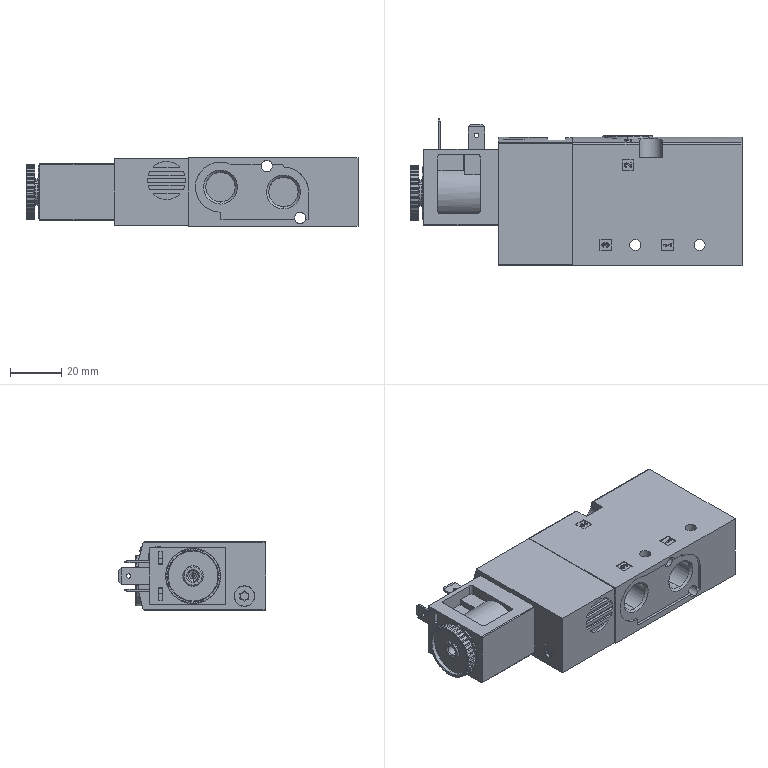Part | SolidWorks | 6 solids | 804 faces | box 129.15 x 57.2 x 26.5 mm | volume 130620 mm3 | plane 357 | cylinder 299 | cone 98 | torus 50 | commonest cylinder face diameters 0.4 x55 1.75 x36 21.5 x36 0.79 x12 1.383 x12 8 x12